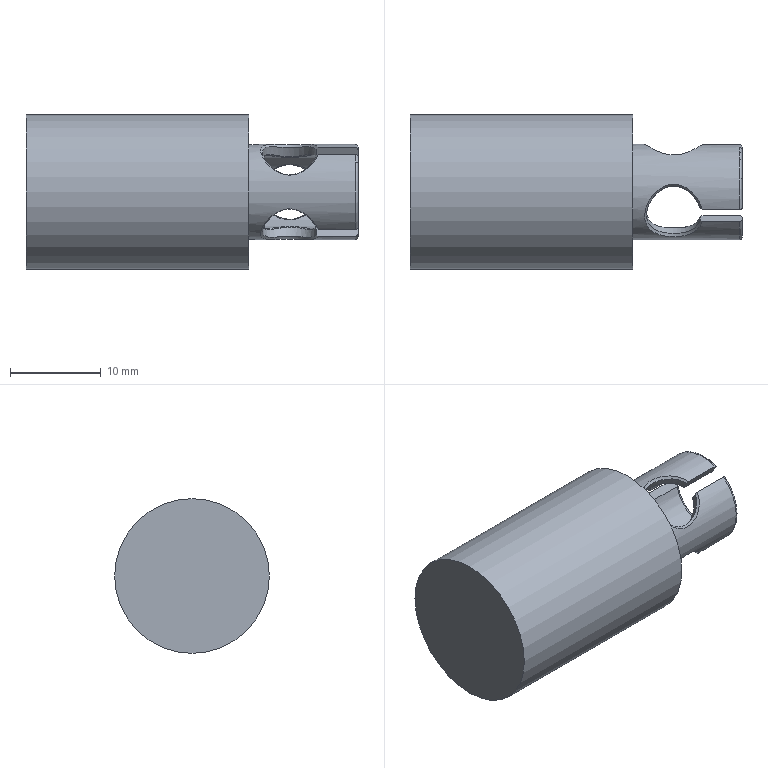Part | STEP file | P0912100001_D | 1 solid | 38 faces | box 36.5 x 17 x 17 mm | volume 4717 mm3 | plane 12 | spline 12 | cylinder 7 | torus 6 | cone 1 | commonest cylinder face diameters 6 x3 8 x1 8.9 x1 10.5 x1 17 x1